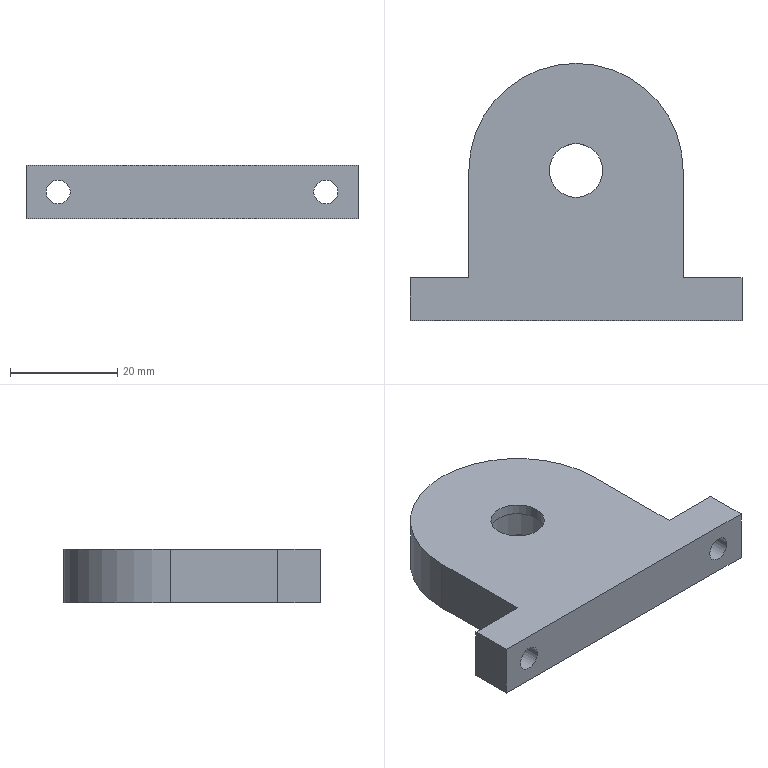Part | Creo | features CURVE 4, CUT 3, DATUM PLANE 3, COORDINATE SYSTEM 1, PROTRUSION 1 | 1 solid | 22 faces | box 62 x 48 x 10 mm | volume 16655 mm3 | plane 11 | cylinder 11 | commonest cylinder face diameters 4.5 x4 10 x2 15.636 x2 19 x2 40 x1
STEP:
#1=CARTESIAN_POINT('',(0.,0.,0.));
#2=DIRECTION('',(0.,0.,1.));
#3=DIRECTION('',(1.,0.,0.));
#4=AXIS2_PLACEMENT_3D('',#1,#2,#3);
#5=CARTESIAN_POINT('',(20.,28.,0.));
#6=VERTEX_POINT('',#5);
#7=CARTESIAN_POINT('',(-20.,28.,0.));
#8=VERTEX_POINT('',#7);
#9=CARTESIAN_POINT('',(0.,28.,0.));
#10=DIRECTION('',(0.,0.,1.));
#11=DIRECTION('',(1.,0.,0.));
#12=AXIS2_PLACEMENT_3D('',#9,#10,#11);
#13=CIRCLE('',#12,20.);
#14=EDGE_CURVE('',#6,#8,#13,.T.);
#15=ORIENTED_EDGE('',*,*,#14,.T.);
#16=CARTESIAN_POINT('',(-20.,8.,0.));
#17=VERTEX_POINT('',#16);
#18=CARTESIAN_POINT('',(-20.,28.,0.));
#19=DIRECTION('',(0.,-1.,0.));
#20=VECTOR('',#19,20.);
#21=LINE('',#18,#20);
#22=EDGE_CURVE('',#8,#17,#21,.T.);
#23=ORIENTED_EDGE('',*,*,#22,.T.);
#24=CARTESIAN_POINT('',(-31.,8.,0.));
#25=VERTEX_POINT('',#24);
#26=CARTESIAN_POINT('',(-20.,8.,0.));
#27=DIRECTION('',(-1.,0.,0.));
#28=VECTOR('',#27,11.);
#29=LINE('',#26,#28);
#30=EDGE_CURVE('',#17,#25,#29,.T.);
#31=ORIENTED_EDGE('',*,*,#30,.T.);
#32=CARTESIAN_POINT('',(-31.,0.,0.));
#33=VERTEX_POINT('',#32);
#34=CARTESIAN_POINT('',(-31.,8.,0.));
#35=DIRECTION('',(0.,-1.,0.));
#36=VECTOR('',#35,8.);
#37=LINE('',#34,#36);
#38=EDGE_CURVE('',#25,#33,#37,.T.);
#39=ORIENTED_EDGE('',*,*,#38,.T.);
#40=CARTESIAN_POINT('',(31.,0.,0.));
#41=VERTEX_POINT('',#40);
#42=CARTESIAN_POINT('',(-31.,0.,0.));
#43=DIRECTION('',(1.,0.,0.));
#44=VECTOR('',#43,62.);
#45=LINE('',#42,#44);
#46=EDGE_CURVE('',#33,#41,#45,.T.);
#47=ORIENTED_EDGE('',*,*,#46,.T.);
#48=CARTESIAN_POINT('',(31.,8.,0.));
#49=VERTEX_POINT('',#48);
#50=CARTESIAN_POINT('',(31.,0.,0.));
#51=DIRECTION('',(0.,1.,0.));
#52=VECTOR('',#51,8.);
#53=LINE('',#50,#52);
#54=EDGE_CURVE('',#41,#49,#53,.T.);
#55=ORIENTED_EDGE('',*,*,#54,.T.);
#56=CARTESIAN_POINT('',(20.,8.,0.));
#57=VERTEX_POINT('',#56);
#58=CARTESIAN_POINT('',(31.,8.,0.));
#59=DIRECTION('',(-1.,0.,0.));
#60=VECTOR('',#59,11.);
#61=LINE('',#58,#60);
#62=EDGE_CURVE('',#49,#57,#61,.T.);
#63=ORIENTED_EDGE('',*,*,#62,.T.);
#64=CARTESIAN_POINT('',(20.,8.,0.));
#65=DIRECTION('',(0.,1.,0.));
#66=VECTOR('',#65,20.);
#67=LINE('',#64,#66);
#68=EDGE_CURVE('',#57,#6,#67,.T.);
#69=ORIENTED_EDGE('',*,*,#68,.T.);
#70=EDGE_LOOP('',(#15,#23,#31,#39,#47,#55,#63,#69));
#71=FACE_OUTER_BOUND('',#70,.F.);
#72=CARTESIAN_POINT('',(-9.5,28.,0.));
#73=VERTEX_POINT('',#72);
#74=CARTESIAN_POINT('',(9.5,28.,0.));
#75=VERTEX_POINT('',#74);
#76=CARTESIAN_POINT('',(0.,28.,0.));
#77=DIRECTION('',(0.,0.,-1.));
#78=DIRECTION('',(-1.,0.,0.));
#79=AXIS2_PLACEMENT_3D('',#76,#77,#78);
#80=CIRCLE('',#79,9.5);
#81=EDGE_CURVE('',#73,#75,#80,.T.);
#82=ORIENTED_EDGE('',*,*,#81,.T.);
#83=CARTESIAN_POINT('',(0.,28.,0.));
#84=DIRECTION('',(0.,0.,-1.));
#85=DIRECTION('',(1.,0.,0.));
#86=AXIS2_PLACEMENT_3D('',#83,#84,#85);
#87=CIRCLE('',#86,9.5);
#88=EDGE_CURVE('',#75,#73,#87,.T.);
#89=ORIENTED_EDGE('',*,*,#88,.T.);
#90=EDGE_LOOP('',(#82,#89));
#91=FACE_BOUND('',#90,.F.);
#92=CARTESIAN_POINT('',(0.,0.,0.));
#93=DIRECTION('',(0.,0.,1.));
#94=DIRECTION('',(1.,0.,0.));
#95=AXIS2_PLACEMENT_3D('',#92,#93,#94);
#96=PLANE('',#95);
#97=ADVANCED_FACE('',(#71,#91),#96,.F.);
#98=ORIENTED_EDGE('',*,*,#14,.F.);
#99=CARTESIAN_POINT('',(20.,28.,10.));
#100=VERTEX_POINT('',#99);
#101=CARTESIAN_POINT('',(20.,28.,0.));
#102=DIRECTION('',(0.,0.,1.));
#103=VECTOR('',#102,10.);
#104=LINE('',#101,#103);
#105=EDGE_CURVE('',#6,#100,#104,.T.);
#106=ORIENTED_EDGE('',*,*,#105,.T.);
#107=CARTESIAN_POINT('',(-20.,28.,10.));
#108=VERTEX_POINT('',#107);
#109=CARTESIAN_POINT('',(0.,28.,10.));
#110=DIRECTION('',(0.,0.,1.));
#111=DIRECTION('',(1.,0.,0.));
#112=AXIS2_PLACEMENT_3D('',#109,#110,#111);
#113=CIRCLE('',#112,20.);
#114=EDGE_CURVE('',#100,#108,#113,.T.);
#115=ORIENTED_EDGE('',*,*,#114,.T.);
#116=CARTESIAN_POINT('',(-20.,28.,0.));
#117=DIRECTION('',(0.,0.,1.));
#118=VECTOR('',#117,10.);
#119=LINE('',#116,#118);
#120=EDGE_CURVE('',#8,#108,#119,.T.);
#121=ORIENTED_EDGE('',*,*,#120,.F.);
#122=EDGE_LOOP('',(#98,#106,#115,#121));
#123=FACE_OUTER_BOUND('',#122,.F.);
#124=CARTESIAN_POINT('',(0.,28.,0.));
#125=DIRECTION('',(0.,0.,1.));
#126=DIRECTION('',(1.,0.,0.));
#127=AXIS2_PLACEMENT_3D('',#124,#125,#126);
#128=CYLINDRICAL_SURFACE('',#127,20.);
#129=ADVANCED_FACE('',(#123),#128,.T.);
#130=ORIENTED_EDGE('',*,*,#68,.F.);
#131=CARTESIAN_POINT('',(20.,8.,10.));
#132=VERTEX_POINT('',#131);
#133=CARTESIAN_POINT('',(20.,8.,0.));
#134=DIRECTION('',(0.,0.,1.));
#135=VECTOR('',#134,10.);
#136=LINE('',#133,#135);
#137=EDGE_CURVE('',#57,#132,#136,.T.);
#138=ORIENTED_EDGE('',*,*,#137,.T.);
#139=CARTESIAN_POINT('',(20.,8.,10.));
#140=DIRECTION('',(0.,1.,0.));
#141=VECTOR('',#140,20.);
#142=LINE('',#139,#141);
#143=EDGE_CURVE('',#132,#100,#142,.T.);
#144=ORIENTED_EDGE('',*,*,#143,.T.);
#145=ORIENTED_EDGE('',*,*,#105,.F.);
#146=EDGE_LOOP('',(#130,#138,#144,#145));
#147=FACE_OUTER_BOUND('',#146,.F.);
#148=CARTESIAN_POINT('',(20.,8.,0.));
#149=DIRECTION('',(1.,0.,0.));
#150=DIRECTION('',(0.,1.,0.));
#151=AXIS2_PLACEMENT_3D('',#148,#149,#150);
#152=PLANE('',#151);
#153=ADVANCED_FACE('',(#147),#152,.T.);
#154=ORIENTED_EDGE('',*,*,#62,.F.);
#155=CARTESIAN_POINT('',(31.,8.,10.));
#156=VERTEX_POINT('',#155);
#157=CARTESIAN_POINT('',(31.,8.,0.));
#158=DIRECTION('',(0.,0.,1.));
#159=VECTOR('',#158,10.);
#160=LINE('',#157,#159);
#161=EDGE_CURVE('',#49,#156,#160,.T.);
#162=ORIENTED_EDGE('',*,*,#161,.T.);
#163=CARTESIAN_POINT('',(31.,8.,10.));
#164=DIRECTION('',(-1.,0.,0.));
#165=VECTOR('',#164,11.);
#166=LINE('',#163,#165);
#167=EDGE_CURVE('',#156,#132,#166,.T.);
#168=ORIENTED_EDGE('',*,*,#167,.T.);
#169=ORIENTED_EDGE('',*,*,#137,.F.);
#170=EDGE_LOOP('',(#154,#162,#168,#169));
#171=FACE_OUTER_BOUND('',#170,.F.);
#172=CARTESIAN_POINT('',(27.25,8.,5.));
#173=VERTEX_POINT('',#172);
#174=CARTESIAN_POINT('',(22.75,8.,5.));
#175=VERTEX_POINT('',#174);
#176=CARTESIAN_POINT('',(25.,8.,5.));
#177=DIRECTION('',(0.,1.,0.));
#178=DIRECTION('',(1.,0.,0.));
#179=AXIS2_PLACEMENT_3D('',#176,#177,#178);
#180=CIRCLE('',#179,2.25);
#181=EDGE_CURVE('',#173,#175,#180,.T.);
#182=ORIENTED_EDGE('',*,*,#181,.T.);
#183=CARTESIAN_POINT('',(25.,8.,5.));
#184=DIRECTION('',(0.,1.,0.));
#185=DIRECTION('',(-1.,0.,0.));
#186=AXIS2_PLACEMENT_3D('',#183,#184,#185);
#187=CIRCLE('',#186,2.25);
#188=EDGE_CURVE('',#175,#173,#187,.T.);
#189=ORIENTED_EDGE('',*,*,#188,.T.);
#190=EDGE_LOOP('',(#182,#189));
#191=FACE_BOUND('',#190,.F.);
#192=CARTESIAN_POINT('',(31.,8.,0.));
#193=DIRECTION('',(0.,1.,0.));
#194=DIRECTION('',(-1.,0.,0.));
#195=AXIS2_PLACEMENT_3D('',#192,#193,#194);
#196=PLANE('',#195);
#197=ADVANCED_FACE('',(#171,#191),#196,.T.);
#198=ORIENTED_EDGE('',*,*,#54,.F.);
#199=CARTESIAN_POINT('',(31.,0.,10.));
#200=VERTEX_POINT('',#199);
#201=CARTESIAN_POINT('',(31.,0.,0.));
#202=DIRECTION('',(0.,0.,1.));
#203=VECTOR('',#202,10.);
#204=LINE('',#201,#203);
#205=EDGE_CURVE('',#41,#200,#204,.T.);
#206=ORIENTED_EDGE('',*,*,#205,.T.);
#207=CARTESIAN_POINT('',(31.,0.,10.));
#208=DIRECTION('',(0.,1.,0.));
#209=VECTOR('',#208,8.);
#210=LINE('',#207,#209);
#211=EDGE_CURVE('',#200,#156,#210,.T.);
#212=ORIENTED_EDGE('',*,*,#211,.T.);
#213=ORIENTED_EDGE('',*,*,#161,.F.);
#214=EDGE_LOOP('',(#198,#206,#212,#213));
#215=FACE_OUTER_BOUND('',#214,.F.);
#216=CARTESIAN_POINT('',(31.,0.,0.));
#217=DIRECTION('',(1.,0.,0.));
#218=DIRECTION('',(0.,1.,0.));
#219=AXIS2_PLACEMENT_3D('',#216,#217,#218);
#220=PLANE('',#219);
#221=ADVANCED_FACE('',(#215),#220,.T.);
#222=ORIENTED_EDGE('',*,*,#46,.F.);
#223=CARTESIAN_POINT('',(-31.,0.,10.));
#224=VERTEX_POINT('',#223);
#225=CARTESIAN_POINT('',(-31.,0.,0.));
#226=DIRECTION('',(0.,0.,1.));
#227=VECTOR('',#226,10.);
#228=LINE('',#225,#227);
#229=EDGE_CURVE('',#33,#224,#228,.T.);
#230=ORIENTED_EDGE('',*,*,#229,.T.);
#231=CARTESIAN_POINT('',(-31.,0.,10.));
#232=DIRECTION('',(1.,0.,0.));
#233=VECTOR('',#232,62.);
#234=LINE('',#231,#233);
#235=EDGE_CURVE('',#224,#200,#234,.T.);
#236=ORIENTED_EDGE('',*,*,#235,.T.);
#237=ORIENTED_EDGE('',*,*,#205,.F.);
#238=EDGE_LOOP('',(#222,#230,#236,#237));
#239=FACE_OUTER_BOUND('',#238,.F.);
#240=CARTESIAN_POINT('',(27.25,0.,5.));
#241=VERTEX_POINT('',#240);
#242=CARTESIAN_POINT('',(22.75,0.,5.));
#243=VERTEX_POINT('',#242);
#244=CARTESIAN_POINT('',(25.,0.,5.));
#245=DIRECTION('',(0.,1.,0.));
#246=DIRECTION('',(1.,0.,0.));
#247=AXIS2_PLACEMENT_3D('',#244,#245,#246);
#248=CIRCLE('',#247,2.25);
#249=EDGE_CURVE('',#241,#243,#248,.T.);
#250=ORIENTED_EDGE('',*,*,#249,.F.);
#251=CARTESIAN_POINT('',(25.,0.,5.));
#252=DIRECTION('',(0.,1.,0.));
#253=DIRECTION('',(-1.,0.,0.));
#254=AXIS2_PLACEMENT_3D('',#251,#252,#253);
#255=CIRCLE('',#254,2.25);
#256=EDGE_CURVE('',#243,#241,#255,.T.);
#257=ORIENTED_EDGE('',*,*,#256,.F.);
#258=EDGE_LOOP('',(#250,#257));
#259=FACE_BOUND('',#258,.F.);
#260=CARTESIAN_POINT('',(-22.75,0.,5.));
#261=VERTEX_POINT('',#260);
#262=CARTESIAN_POINT('',(-27.25,0.,5.));
#263=VERTEX_POINT('',#262);
#264=CARTESIAN_POINT('',(-25.,0.,5.));
#265=DIRECTION('',(0.,1.,0.));
#266=DIRECTION('',(1.,0.,0.));
#267=AXIS2_PLACEMENT_3D('',#264,#265,#266);
#268=CIRCLE('',#267,2.25);
#269=EDGE_CURVE('',#261,#263,#268,.T.);
#270=ORIENTED_EDGE('',*,*,#269,.F.);
#271=CARTESIAN_POINT('',(-25.,0.,5.));
#272=DIRECTION('',(0.,1.,0.));
#273=DIRECTION('',(-1.,0.,0.));
#274=AXIS2_PLACEMENT_3D('',#271,#272,#273);
#275=CIRCLE('',#274,2.25);
#276=EDGE_CURVE('',#263,#261,#275,.T.);
#277=ORIENTED_EDGE('',*,*,#276,.F.);
#278=EDGE_LOOP('',(#270,#277));
#279=FACE_BOUND('',#278,.F.);
#280=CARTESIAN_POINT('',(-31.,0.,0.));
#281=DIRECTION('',(0.,-1.,0.));
#282=DIRECTION('',(1.,0.,0.));
#283=AXIS2_PLACEMENT_3D('',#280,#281,#282);
#284=PLANE('',#283);
#285=ADVANCED_FACE('',(#239,#259,#279),#284,.T.);
#286=ORIENTED_EDGE('',*,*,#38,.F.);
#287=CARTESIAN_POINT('',(-31.,8.,10.));
#288=VERTEX_POINT('',#287);
#289=CARTESIAN_POINT('',(-31.,8.,0.));
#290=DIRECTION('',(0.,0.,1.));
#291=VECTOR('',#290,10.);
#292=LINE('',#289,#291);
#293=EDGE_CURVE('',#25,#288,#292,.T.);
#294=ORIENTED_EDGE('',*,*,#293,.T.);
#295=CARTESIAN_POINT('',(-31.,8.,10.));
#296=DIRECTION('',(0.,-1.,0.));
#297=VECTOR('',#296,8.);
#298=LINE('',#295,#297);
#299=EDGE_CURVE('',#288,#224,#298,.T.);
#300=ORIENTED_EDGE('',*,*,#299,.T.);
#301=ORIENTED_EDGE('',*,*,#229,.F.);
#302=EDGE_LOOP('',(#286,#294,#300,#301));
#303=FACE_OUTER_BOUND('',#302,.F.);
#304=CARTESIAN_POINT('',(-31.,8.,0.));
#305=DIRECTION('',(-1.,0.,0.));
#306=DIRECTION('',(0.,-1.,0.));
#307=AXIS2_PLACEMENT_3D('',#304,#305,#306);
#308=PLANE('',#307);
#309=ADVANCED_FACE('',(#303),#308,.T.);
#310=ORIENTED_EDGE('',*,*,#30,.F.);
#311=CARTESIAN_POINT('',(-20.,8.,10.));
#312=VERTEX_POINT('',#311);
#313=CARTESIAN_POINT('',(-20.,8.,0.));
#314=DIRECTION('',(0.,0.,1.));
#315=VECTOR('',#314,10.);
#316=LINE('',#313,#315);
#317=EDGE_CURVE('',#17,#312,#316,.T.);
#318=ORIENTED_EDGE('',*,*,#317,.T.);
#319=CARTESIAN_POINT('',(-20.,8.,10.));
#320=DIRECTION('',(-1.,0.,0.));
#321=VECTOR('',#320,11.);
#322=LINE('',#319,#321);
#323=EDGE_CURVE('',#312,#288,#322,.T.);
#324=ORIENTED_EDGE('',*,*,#323,.T.);
#325=ORIENTED_EDGE('',*,*,#293,.F.);
#326=EDGE_LOOP('',(#310,#318,#324,#325));
#327=FACE_OUTER_BOUND('',#326,.F.);
#328=CARTESIAN_POINT('',(-22.75,8.,5.));
#329=VERTEX_POINT('',#328);
#330=CARTESIAN_POINT('',(-27.25,8.,5.));
#331=VERTEX_POINT('',#330);
#332=CARTESIAN_POINT('',(-25.,8.,5.));
#333=DIRECTION('',(0.,1.,0.));
#334=DIRECTION('',(1.,0.,0.));
#335=AXIS2_PLACEMENT_3D('',#332,#333,#334);
#336=CIRCLE('',#335,2.25);
#337=EDGE_CURVE('',#329,#331,#336,.T.);
#338=ORIENTED_EDGE('',*,*,#337,.T.);
#339=CARTESIAN_POINT('',(-25.,8.,5.));
#340=DIRECTION('',(0.,1.,0.));
#341=DIRECTION('',(-1.,0.,0.));
#342=AXIS2_PLACEMENT_3D('',#339,#340,#341);
#343=CIRCLE('',#342,2.25);
#344=EDGE_CURVE('',#331,#329,#343,.T.);
#345=ORIENTED_EDGE('',*,*,#344,.T.);
#346=EDGE_LOOP('',(#338,#345));
#347=FACE_BOUND('',#346,.F.);
#348=CARTESIAN_POINT('',(-20.,8.,0.));
#349=DIRECTION('',(0.,1.,0.));
#350=DIRECTION('',(-1.,0.,0.));
#351=AXIS2_PLACEMENT_3D('',#348,#349,#350);
#352=PLANE('',#351);
#353=ADVANCED_FACE('',(#327,#347),#352,.T.);
#354=ORIENTED_EDGE('',*,*,#22,.F.);
#355=ORIENTED_EDGE('',*,*,#120,.T.);
#356=CARTESIAN_POINT('',(-20.,28.,10.));
#357=DIRECTION('',(0.,-1.,0.));
#358=VECTOR('',#357,20.);
#359=LINE('',#356,#358);
#360=EDGE_CURVE('',#108,#312,#359,.T.);
#361=ORIENTED_EDGE('',*,*,#360,.T.);
#362=ORIENTED_EDGE('',*,*,#317,.F.);
#363=EDGE_LOOP('',(#354,#355,#361,#362));
#364=FACE_OUTER_BOUND('',#363,.F.);
#365=CARTESIAN_POINT('',(-20.,28.,0.));
#366=DIRECTION('',(-1.,0.,0.));
#367=DIRECTION('',(0.,-1.,0.));
#368=AXIS2_PLACEMENT_3D('',#365,#366,#367);
#369=PLANE('',#368);
#370=ADVANCED_FACE('',(#364),#369,.T.);
#371=ORIENTED_EDGE('',*,*,#114,.F.);
#372=ORIENTED_EDGE('',*,*,#143,.F.);
#373=ORIENTED_EDGE('',*,*,#167,.F.);
#374=ORIENTED_EDGE('',*,*,#211,.F.);
#375=ORIENTED_EDGE('',*,*,#235,.F.);
#376=ORIENTED_EDGE('',*,*,#299,.F.);
#377=ORIENTED_EDGE('',*,*,#323,.F.);
#378=ORIENTED_EDGE('',*,*,#360,.F.);
#379=EDGE_LOOP('',(#371,#372,#373,#374,#375,#376,#377,#378));
#380=FACE_OUTER_BOUND('',#379,.F.);
#381=CARTESIAN_POINT('',(5.,28.,10.));
#382=VERTEX_POINT('',#381);
#383=CARTESIAN_POINT('',(-5.,28.,10.));
#384=VERTEX_POINT('',#383);
#385=CARTESIAN_POINT('',(0.,28.,10.));
#386=DIRECTION('',(0.,0.,-1.));
#387=DIRECTION('',(1.,0.,0.));
#388=AXIS2_PLACEMENT_3D('',#385,#386,#387);
#389=CIRCLE('',#388,5.);
#390=EDGE_CURVE('',#382,#384,#389,.T.);
#391=ORIENTED_EDGE('',*,*,#390,.F.);
#392=CARTESIAN_POINT('',(0.,28.,10.));
#393=DIRECTION('',(0.,0.,-1.));
#394=DIRECTION('',(-1.,0.,0.));
#395=AXIS2_PLACEMENT_3D('',#392,#393,#394);
#396=CIRCLE('',#395,5.);
#397=EDGE_CURVE('',#384,#382,#396,.T.);
#398=ORIENTED_EDGE('',*,*,#397,.F.);
#399=EDGE_LOOP('',(#391,#398));
#400=FACE_BOUND('',#399,.F.);
#401=CARTESIAN_POINT('',(0.,0.,10.));
#402=DIRECTION('',(0.,0.,1.));
#403=DIRECTION('',(1.,0.,0.));
#404=AXIS2_PLACEMENT_3D('',#401,#402,#403);
#405=PLANE('',#404);
#406=ADVANCED_FACE('',(#380,#400),#405,.T.);
#407=CARTESIAN_POINT('',(-5.,28.,8.));
#408=VERTEX_POINT('',#407);
#409=CARTESIAN_POINT('',(5.,28.,8.));
#410=VERTEX_POINT('',#409);
#411=CARTESIAN_POINT('',(0.,28.,8.));
#412=DIRECTION('',(0.,0.,1.));
#413=DIRECTION('',(-1.,0.,0.));
#414=AXIS2_PLACEMENT_3D('',#411,#412,#413);
#415=CIRCLE('',#414,5.);
#416=EDGE_CURVE('',#408,#410,#415,.T.);
#417=ORIENTED_EDGE('',*,*,#416,.T.);
#418=CARTESIAN_POINT('',(5.,28.,8.));
#419=DIRECTION('',(0.,0.,1.));
#420=VECTOR('',#419,2.);
#421=LINE('',#418,#420);
#422=EDGE_CURVE('',#410,#382,#421,.T.);
#423=ORIENTED_EDGE('',*,*,#422,.T.);
#424=ORIENTED_EDGE('',*,*,#390,.T.);
#425=CARTESIAN_POINT('',(-5.,28.,8.));
#426=DIRECTION('',(0.,0.,1.));
#427=VECTOR('',#426,2.);
#428=LINE('',#425,#427);
#429=EDGE_CURVE('',#408,#384,#428,.T.);
#430=ORIENTED_EDGE('',*,*,#429,.F.);
#431=EDGE_LOOP('',(#417,#423,#424,#430));
#432=FACE_OUTER_BOUND('',#431,.F.);
#433=CARTESIAN_POINT('',(0.,28.,0.));
#434=DIRECTION('',(0.,0.,1.));
#435=DIRECTION('',(1.,0.,0.));
#436=AXIS2_PLACEMENT_3D('',#433,#434,#435);
#437=CYLINDRICAL_SURFACE('',#436,5.);
#438=ADVANCED_FACE('',(#432),#437,.F.);
#439=CARTESIAN_POINT('',(-7.818,28.,8.));
#440=VERTEX_POINT('',#439);
#441=CARTESIAN_POINT('',(7.818,28.,8.));
#442=VERTEX_POINT('',#441);
#443=CARTESIAN_POINT('',(0.,28.,8.));
#444=DIRECTION('',(0.,0.,-1.));
#445=DIRECTION('',(-1.,0.,0.));
#446=AXIS2_PLACEMENT_3D('',#443,#444,#445);
#447=CIRCLE('',#446,7.818);
#448=EDGE_CURVE('',#440,#442,#447,.T.);
#449=ORIENTED_EDGE('',*,*,#448,.F.);
#450=CARTESIAN_POINT('',(0.,28.,8.));
#451=DIRECTION('',(0.,0.,-1.));
#452=DIRECTION('',(1.,0.,0.));
#453=AXIS2_PLACEMENT_3D('',#450,#451,#452);
#454=CIRCLE('',#453,7.818);
#455=EDGE_CURVE('',#442,#440,#454,.T.);
#456=ORIENTED_EDGE('',*,*,#455,.F.);
#457=EDGE_LOOP('',(#449,#456));
#458=FACE_OUTER_BOUND('',#457,.F.);
#459=ORIENTED_EDGE('',*,*,#416,.F.);
#460=CARTESIAN_POINT('',(0.,28.,8.));
#461=DIRECTION('',(0.,0.,1.));
#462=DIRECTION('',(1.,0.,0.));
#463=AXIS2_PLACEMENT_3D('',#460,#461,#462);
#464=CIRCLE('',#463,5.);
#465=EDGE_CURVE('',#410,#408,#464,.T.);
#466=ORIENTED_EDGE('',*,*,#465,.F.);
#467=EDGE_LOOP('',(#459,#466));
#468=FACE_BOUND('',#467,.F.);
#469=CARTESIAN_POINT('',(0.,0.,8.));
#470=DIRECTION('',(0.,0.,-1.));
#471=DIRECTION('',(-1.,0.,0.));
#472=AXIS2_PLACEMENT_3D('',#469,#470,#471);
#473=PLANE('',#472);
#474=ADVANCED_FACE('',(#458,#468),#473,.T.);
#475=CARTESIAN_POINT('',(-7.818,28.,7.));
#476=VERTEX_POINT('',#475);
#477=CARTESIAN_POINT('',(7.818,28.,7.));
#478=VERTEX_POINT('',#477);
#479=CARTESIAN_POINT('',(0.,28.,7.));
#480=DIRECTION('',(0.,0.,-1.));
#481=DIRECTION('',(-1.,0.,0.));
#482=AXIS2_PLACEMENT_3D('',#479,#480,#481);
#483=CIRCLE('',#482,7.818);
#484=EDGE_CURVE('',#476,#478,#483,.T.);
#485=ORIENTED_EDGE('',*,*,#484,.F.);
#486=CARTESIAN_POINT('',(-7.818,28.,7.));
#487=DIRECTION('',(0.,0.,1.));
#488=VECTOR('',#487,1.);
#489=LINE('',#486,#488);
#490=EDGE_CURVE('',#476,#440,#489,.T.);
#491=ORIENTED_EDGE('',*,*,#490,.T.);
#492=ORIENTED_EDGE('',*,*,#448,.T.);
#493=CARTESIAN_POINT('',(7.818,28.,7.));
#494=DIRECTION('',(0.,0.,1.));
#495=VECTOR('',#494,1.);
#496=LINE('',#493,#495);
#497=EDGE_CURVE('',#478,#442,#496,.T.);
#498=ORIENTED_EDGE('',*,*,#497,.F.);
#499=EDGE_LOOP('',(#485,#491,#492,#498));
#500=FACE_OUTER_BOUND('',#499,.F.);
#501=CARTESIAN_POINT('',(0.,28.,7.));
#502=DIRECTION('',(0.,0.,-1.));
#503=DIRECTION('',(-1.,0.,0.));
#504=AXIS2_PLACEMENT_3D('',#501,#502,#503);
#505=CYLINDRICAL_SURFACE('',#504,7.818);
#506=ADVANCED_FACE('',(#500),#505,.F.);
#507=CARTESIAN_POINT('',(-9.5,28.,7.));
#508=VERTEX_POINT('',#507);
#509=CARTESIAN_POINT('',(9.5,28.,7.));
#510=VERTEX_POINT('',#509);
#511=CARTESIAN_POINT('',(0.,28.,7.));
#512=DIRECTION('',(0.,0.,-1.));
#513=DIRECTION('',(-1.,0.,0.));
#514=AXIS2_PLACEMENT_3D('',#511,#512,#513);
#515=CIRCLE('',#514,9.5);
#516=EDGE_CURVE('',#508,#510,#515,.T.);
#517=ORIENTED_EDGE('',*,*,#516,.F.);
#518=CARTESIAN_POINT('',(0.,28.,7.));
#519=DIRECTION('',(0.,0.,-1.));
#520=DIRECTION('',(1.,0.,0.));
#521=AXIS2_PLACEMENT_3D('',#518,#519,#520);
#522=CIRCLE('',#521,9.5);
#523=EDGE_CURVE('',#510,#508,#522,.T.);
#524=ORIENTED_EDGE('',*,*,#523,.F.);
#525=EDGE_LOOP('',(#517,#524));
#526=FACE_OUTER_BOUND('',#525,.F.);
#527=ORIENTED_EDGE('',*,*,#484,.T.);
#528=CARTESIAN_POINT('',(0.,28.,7.));
#529=DIRECTION('',(0.,0.,-1.));
#530=DIRECTION('',(1.,0.,0.));
#531=AXIS2_PLACEMENT_3D('',#528,#529,#530);
#532=CIRCLE('',#531,7.818);
#533=EDGE_CURVE('',#478,#476,#532,.T.);
#534=ORIENTED_EDGE('',*,*,#533,.T.);
#535=EDGE_LOOP('',(#527,#534));
#536=FACE_BOUND('',#535,.F.);
#537=CARTESIAN_POINT('',(0.,0.,7.));
#538=DIRECTION('',(0.,0.,-1.));
#539=DIRECTION('',(-1.,0.,0.));
#540=AXIS2_PLACEMENT_3D('',#537,#538,#539);
#541=PLANE('',#540);
#542=ADVANCED_FACE('',(#526,#536),#541,.T.);
#543=ORIENTED_EDGE('',*,*,#81,.F.);
#544=CARTESIAN_POINT('',(-9.5,28.,0.));
#545=DIRECTION('',(0.,0.,1.));
#546=VECTOR('',#545,7.);
#547=LINE('',#544,#546);
#548=EDGE_CURVE('',#73,#508,#547,.T.);
#549=ORIENTED_EDGE('',*,*,#548,.T.);
#550=ORIENTED_EDGE('',*,*,#516,.T.);
#551=CARTESIAN_POINT('',(9.5,28.,0.));
#552=DIRECTION('',(0.,0.,1.));
#553=VECTOR('',#552,7.);
#554=LINE('',#551,#553);
#555=EDGE_CURVE('',#75,#510,#554,.T.);
#556=ORIENTED_EDGE('',*,*,#555,.F.);
#557=EDGE_LOOP('',(#543,#549,#550,#556));
#558=FACE_OUTER_BOUND('',#557,.F.);
#559=CARTESIAN_POINT('',(0.,28.,0.));
#560=DIRECTION('',(0.,0.,-1.));
#561=DIRECTION('',(-1.,0.,0.));
#562=AXIS2_PLACEMENT_3D('',#559,#560,#561);
#563=CYLINDRICAL_SURFACE('',#562,9.5);
#564=ADVANCED_FACE('',(#558),#563,.F.);
#565=ORIENTED_EDGE('',*,*,#88,.F.);
#566=ORIENTED_EDGE('',*,*,#555,.T.);
#567=ORIENTED_EDGE('',*,*,#523,.T.);
#568=ORIENTED_EDGE('',*,*,#548,.F.);
#569=EDGE_LOOP('',(#565,#566,#567,#568));
#570=FACE_OUTER_BOUND('',#569,.F.);
#571=CARTESIAN_POINT('',(0.,28.,0.));
#572=DIRECTION('',(0.,0.,-1.));
#573=DIRECTION('',(-1.,0.,0.));
#574=AXIS2_PLACEMENT_3D('',#571,#572,#573);
#575=CYLINDRICAL_SURFACE('',#574,9.5);
#576=ADVANCED_FACE('',(#570),#575,.F.);
#577=ORIENTED_EDGE('',*,*,#533,.F.);
#578=ORIENTED_EDGE('',*,*,#497,.T.);
#579=ORIENTED_EDGE('',*,*,#455,.T.);
#580=ORIENTED_EDGE('',*,*,#490,.F.);
#581=EDGE_LOOP('',(#577,#578,#579,#580));
#582=FACE_OUTER_BOUND('',#581,.F.);
#583=CARTESIAN_POINT('',(0.,28.,7.));
#584=DIRECTION('',(0.,0.,-1.));
#585=DIRECTION('',(-1.,0.,0.));
#586=AXIS2_PLACEMENT_3D('',#583,#584,#585);
#587=CYLINDRICAL_SURFACE('',#586,7.818);
#588=ADVANCED_FACE('',(#582),#587,.F.);
#589=ORIENTED_EDGE('',*,*,#465,.T.);
#590=ORIENTED_EDGE('',*,*,#429,.T.);
#591=ORIENTED_EDGE('',*,*,#397,.T.);
#592=ORIENTED_EDGE('',*,*,#422,.F.);
#593=EDGE_LOOP('',(#589,#590,#591,#592));
#594=FACE_OUTER_BOUND('',#593,.F.);
#595=CARTESIAN_POINT('',(0.,28.,0.));
#596=DIRECTION('',(0.,0.,1.));
#597=DIRECTION('',(1.,0.,0.));
#598=AXIS2_PLACEMENT_3D('',#595,#596,#597);
#599=CYLINDRICAL_SURFACE('',#598,5.);
#600=ADVANCED_FACE('',(#594),#599,.F.);
#601=ORIENTED_EDGE('',*,*,#337,.F.);
#602=CARTESIAN_POINT('',(-22.75,8.,5.));
#603=DIRECTION('',(0.,-1.,0.));
#604=VECTOR('',#603,8.);
#605=LINE('',#602,#604);
#606=EDGE_CURVE('',#329,#261,#605,.T.);
#607=ORIENTED_EDGE('',*,*,#606,.T.);
#608=ORIENTED_EDGE('',*,*,#269,.T.);
#609=CARTESIAN_POINT('',(-27.25,8.,5.));
#610=DIRECTION('',(0.,-1.,0.));
#611=VECTOR('',#610,8.);
#612=LINE('',#609,#611);
#613=EDGE_CURVE('',#331,#263,#612,.T.);
#614=ORIENTED_EDGE('',*,*,#613,.F.);
#615=EDGE_LOOP('',(#601,#607,#608,#614));
#616=FACE_OUTER_BOUND('',#615,.F.);
#617=CARTESIAN_POINT('',(-25.,8.,5.));
#618=DIRECTION('',(0.,1.,0.));
#619=DIRECTION('',(1.,0.,0.));
#620=AXIS2_PLACEMENT_3D('',#617,#618,#619);
#621=CYLINDRICAL_SURFACE('',#620,2.25);
#622=ADVANCED_FACE('',(#616),#621,.F.);
#623=ORIENTED_EDGE('',*,*,#344,.F.);
#624=ORIENTED_EDGE('',*,*,#613,.T.);
#625=ORIENTED_EDGE('',*,*,#276,.T.);
#626=ORIENTED_EDGE('',*,*,#606,.F.);
#627=EDGE_LOOP('',(#623,#624,#625,#626));
#628=FACE_OUTER_BOUND('',#627,.F.);
#629=CARTESIAN_POINT('',(-25.,8.,5.));
#630=DIRECTION('',(0.,1.,0.));
#631=DIRECTION('',(1.,0.,0.));
#632=AXIS2_PLACEMENT_3D('',#629,#630,#631);
#633=CYLINDRICAL_SURFACE('',#632,2.25);
#634=ADVANCED_FACE('',(#628),#633,.F.);
#635=ORIENTED_EDGE('',*,*,#249,.T.);
#636=CARTESIAN_POINT('',(22.75,8.,5.));
#637=DIRECTION('',(0.,-1.,0.));
#638=VECTOR('',#637,8.);
#639=LINE('',#636,#638);
#640=EDGE_CURVE('',#175,#243,#639,.T.);
#641=ORIENTED_EDGE('',*,*,#640,.F.);
#642=ORIENTED_EDGE('',*,*,#181,.F.);
#643=CARTESIAN_POINT('',(27.25,8.,5.));
#644=DIRECTION('',(0.,-1.,0.));
#645=VECTOR('',#644,8.);
#646=LINE('',#643,#645);
#647=EDGE_CURVE('',#173,#241,#646,.T.);
#648=ORIENTED_EDGE('',*,*,#647,.T.);
#649=EDGE_LOOP('',(#635,#641,#642,#648));
#650=FACE_OUTER_BOUND('',#649,.F.);
#651=CARTESIAN_POINT('',(25.,8.,5.));
#652=DIRECTION('',(0.,1.,0.));
#653=DIRECTION('',(1.,0.,0.));
#654=AXIS2_PLACEMENT_3D('',#651,#652,#653);
#655=CYLINDRICAL_SURFACE('',#654,2.25);
#656=ADVANCED_FACE('',(#650),#655,.F.);
#657=ORIENTED_EDGE('',*,*,#256,.T.);
#658=ORIENTED_EDGE('',*,*,#647,.F.);
#659=ORIENTED_EDGE('',*,*,#188,.F.);
#660=ORIENTED_EDGE('',*,*,#640,.T.);
#661=EDGE_LOOP('',(#657,#658,#659,#660));
#662=FACE_OUTER_BOUND('',#661,.F.);
#663=CARTESIAN_POINT('',(25.,8.,5.));
#664=DIRECTION('',(0.,1.,0.));
#665=DIRECTION('',(1.,0.,0.));
#666=AXIS2_PLACEMENT_3D('',#663,#664,#665);
#667=CYLINDRICAL_SURFACE('',#666,2.25);
#668=ADVANCED_FACE('',(#662),#667,.F.);
#669=CLOSED_SHELL('',(#97,#129,#153,#197,#221,#285,#309,#353,#370,#406,#438,#474,#506,#542,#564,#576,#588,#600,#622,#634,#656,#668));
#670=MANIFOLD_SOLID_BREP('',#669);
#671=(LENGTH_UNIT()NAMED_UNIT(*)SI_UNIT(.MILLI.,.METRE.));
#672=UNCERTAINTY_MEASURE_WITH_UNIT(LENGTH_MEASURE(0.007904),#671,'','');
#673=(NAMED_UNIT(*)PLANE_ANGLE_UNIT()SI_UNIT($,.RADIAN.));
#674=PLANE_ANGLE_MEASURE_WITH_UNIT(PLANE_ANGLE_MEASURE(0.01745),#673);
#675=(CONVERSION_BASED_UNIT('DEGREE',#674)NAMED_UNIT(*)PLANE_ANGLE_UNIT());
#676=(NAMED_UNIT(*)SI_UNIT($,.STERADIAN.)SOLID_ANGLE_UNIT());
#677=(GEOMETRIC_REPRESENTATION_CONTEXT(3)GLOBAL_UNCERTAINTY_ASSIGNED_CONTEXT((#672))GLOBAL_UNIT_ASSIGNED_CONTEXT((#671,#675,#676))REPRESENTATION_CONTEXT('',''));
#678=ADVANCED_BREP_SHAPE_REPRESENTATION('',(#4,#670),#677);